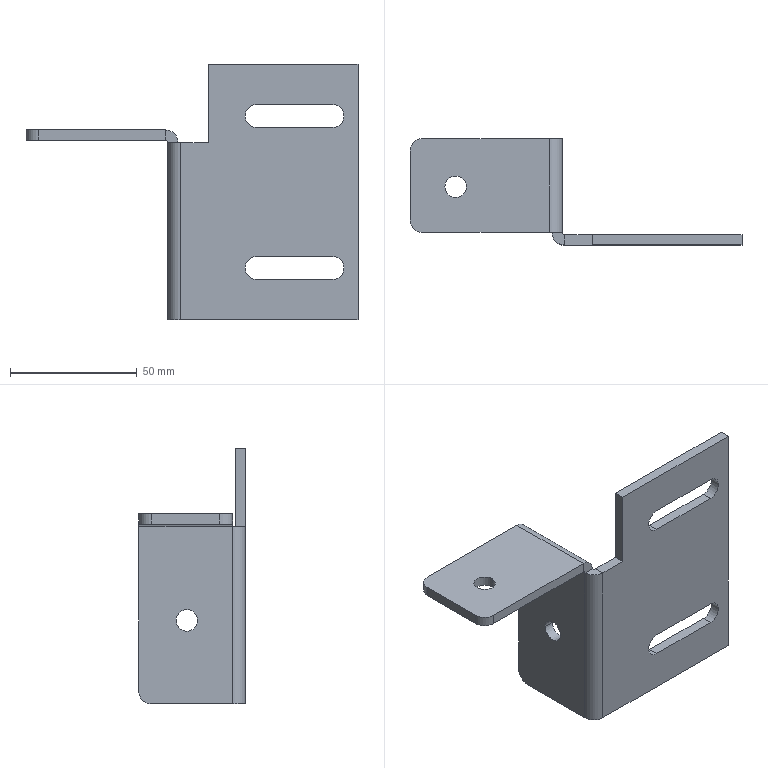Part | 1 solid | 39 faces | box 131 x 42 x 101 mm | volume 44246 mm3 | plane 24 | cylinder 15 | commonest cylinder face diameters 10 x5 8.5 x4 9 x4 2 x2
STEP:
#1=CARTESIAN_POINT('',(-24.207,-9.491,33.));
#2=VERTEX_POINT('',#1);
#3=CARTESIAN_POINT('',(-24.207,-0.9914,33.));
#4=VERTEX_POINT('',#3);
#5=CARTESIAN_POINT('',(-24.207,-5.241,33.));
#6=DIRECTION('',(1.,0.,0.));
#7=DIRECTION('',(0.,1.,0.));
#8=AXIS2_PLACEMENT_3D('',#5,#6,#7);
#9=CIRCLE('',#8,4.25);
#10=EDGE_CURVE('',#2,#4,#9,.T.);
#11=ORIENTED_EDGE('',*,*,#10,.F.);
#12=CARTESIAN_POINT('',(-20.207,-9.491,33.));
#13=VERTEX_POINT('',#12);
#14=CARTESIAN_POINT('',(-30.207,-9.491,33.));
#15=DIRECTION('',(1.,0.,0.));
#16=VECTOR('',#15,1000.);
#17=LINE('',#14,#16);
#18=EDGE_CURVE('',#2,#13,#17,.T.);
#19=ORIENTED_EDGE('',*,*,#18,.T.);
#20=CARTESIAN_POINT('',(-20.207,-0.9914,33.));
#21=VERTEX_POINT('',#20);
#22=CARTESIAN_POINT('',(-20.207,-5.241,33.));
#23=DIRECTION('',(1.,0.,0.));
#24=DIRECTION('',(0.,1.,0.));
#25=AXIS2_PLACEMENT_3D('',#22,#23,#24);
#26=CIRCLE('',#25,4.25);
#27=EDGE_CURVE('',#13,#21,#26,.T.);
#28=ORIENTED_EDGE('',*,*,#27,.T.);
#29=CARTESIAN_POINT('',(-30.207,-0.9914,33.));
#30=DIRECTION('',(1.,0.,0.));
#31=VECTOR('',#30,1000.);
#32=LINE('',#29,#31);
#33=EDGE_CURVE('',#4,#21,#32,.T.);
#34=ORIENTED_EDGE('',*,*,#33,.F.);
#35=EDGE_LOOP('',(#11,#19,#28,#34));
#36=FACE_OUTER_BOUND('',#35,.T.);
#37=CARTESIAN_POINT('',(-30.207,-5.241,33.));
#38=DIRECTION('',(1.,0.,0.));
#39=DIRECTION('',(0.,1.,0.));
#40=AXIS2_PLACEMENT_3D('',#37,#38,#39);
#41=CYLINDRICAL_SURFACE('',#40,4.25);
#42=ADVANCED_FACE('',(#36),#41,.F.);
#43=CARTESIAN_POINT('',(-66.457,-5.241,71.));
#44=VERTEX_POINT('',#43);
#45=CARTESIAN_POINT('',(-57.957,-5.241,71.));
#46=VERTEX_POINT('',#45);
#47=CARTESIAN_POINT('',(-62.207,-5.241,71.));
#48=DIRECTION('',(0.,0.,1.));
#49=DIRECTION('',(1.,0.,0.));
#50=AXIS2_PLACEMENT_3D('',#47,#48,#49);
#51=CIRCLE('',#50,4.25);
#52=EDGE_CURVE('',#44,#46,#51,.T.);
#53=ORIENTED_EDGE('',*,*,#52,.F.);
#54=CARTESIAN_POINT('',(-66.457,-5.241,75.));
#55=VERTEX_POINT('',#54);
#56=CARTESIAN_POINT('',(-66.457,-5.241,65.));
#57=DIRECTION('',(0.,0.,1.));
#58=VECTOR('',#57,1000.);
#59=LINE('',#56,#58);
#60=EDGE_CURVE('',#44,#55,#59,.T.);
#61=ORIENTED_EDGE('',*,*,#60,.T.);
#62=CARTESIAN_POINT('',(-57.957,-5.241,75.));
#63=VERTEX_POINT('',#62);
#64=CARTESIAN_POINT('',(-62.207,-5.241,75.));
#65=DIRECTION('',(0.,0.,1.));
#66=DIRECTION('',(1.,0.,0.));
#67=AXIS2_PLACEMENT_3D('',#64,#65,#66);
#68=CIRCLE('',#67,4.25);
#69=EDGE_CURVE('',#55,#63,#68,.T.);
#70=ORIENTED_EDGE('',*,*,#69,.T.);
#71=CARTESIAN_POINT('',(-57.957,-5.241,65.));
#72=DIRECTION('',(0.,0.,1.));
#73=VECTOR('',#72,1000.);
#74=LINE('',#71,#73);
#75=EDGE_CURVE('',#46,#63,#74,.T.);
#76=ORIENTED_EDGE('',*,*,#75,.F.);
#77=EDGE_LOOP('',(#53,#61,#70,#76));
#78=FACE_OUTER_BOUND('',#77,.T.);
#79=CARTESIAN_POINT('',(-62.207,-5.241,65.));
#80=DIRECTION('',(0.,0.,1.));
#81=DIRECTION('',(1.,0.,0.));
#82=AXIS2_PLACEMENT_3D('',#79,#80,#81);
#83=CYLINDRICAL_SURFACE('',#82,4.25);
#84=ADVANCED_FACE('',(#78),#83,.F.);
#85=CARTESIAN_POINT('',(-8.207,-24.241,70.));
#86=VERTEX_POINT('',#85);
#87=CARTESIAN_POINT('',(-19.207,-24.241,70.));
#88=VERTEX_POINT('',#87);
#89=CARTESIAN_POINT('',(-24.207,-24.241,70.));
#90=DIRECTION('',(-1.,0.,0.));
#91=VECTOR('',#90,1000.);
#92=LINE('',#89,#91);
#93=EDGE_CURVE('',#86,#88,#92,.T.);
#94=ORIENTED_EDGE('',*,*,#93,.T.);
#95=CARTESIAN_POINT('',(-19.207,-28.241,70.));
#96=VERTEX_POINT('',#95);
#97=CARTESIAN_POINT('',(-19.207,-24.241,70.));
#98=DIRECTION('',(0.,-1.,0.));
#99=VECTOR('',#98,1000.);
#100=LINE('',#97,#99);
#101=EDGE_CURVE('',#88,#96,#100,.T.);
#102=ORIENTED_EDGE('',*,*,#101,.T.);
#103=CARTESIAN_POINT('',(-8.207,-28.241,70.));
#104=VERTEX_POINT('',#103);
#105=CARTESIAN_POINT('',(-8.207,-28.241,70.));
#106=DIRECTION('',(-1.,0.,0.));
#107=VECTOR('',#106,1000.);
#108=LINE('',#105,#107);
#109=EDGE_CURVE('',#104,#96,#108,.T.);
#110=ORIENTED_EDGE('',*,*,#109,.F.);
#111=CARTESIAN_POINT('',(-8.207,-28.241,70.));
#112=DIRECTION('',(0.,1.,0.));
#113=VECTOR('',#112,1000.);
#114=LINE('',#111,#113);
#115=EDGE_CURVE('',#104,#86,#114,.T.);
#116=ORIENTED_EDGE('',*,*,#115,.T.);
#117=EDGE_LOOP('',(#94,#102,#110,#116));
#118=FACE_OUTER_BOUND('',#117,.T.);
#119=CARTESIAN_POINT('',(-8.207,-28.241,70.));
#120=DIRECTION('',(0.,0.,-1.));
#121=DIRECTION('',(-1.,0.,0.));
#122=AXIS2_PLACEMENT_3D('',#119,#120,#121);
#123=PLANE('',#122);
#124=ADVANCED_FACE('',(#118),#123,.F.);
#125=CARTESIAN_POINT('',(-19.207,-28.241,0.));
#126=VERTEX_POINT('',#125);
#127=CARTESIAN_POINT('',(-19.207,-24.241,0.));
#128=VERTEX_POINT('',#127);
#129=CARTESIAN_POINT('',(-19.207,-28.241,0.));
#130=DIRECTION('',(0.,1.,0.));
#131=VECTOR('',#130,1000.);
#132=LINE('',#129,#131);
#133=EDGE_CURVE('',#126,#128,#132,.T.);
#134=ORIENTED_EDGE('',*,*,#133,.F.);
#135=CARTESIAN_POINT('',(-24.207,-23.241,0.));
#136=VERTEX_POINT('',#135);
#137=CARTESIAN_POINT('',(-19.207,-23.241,0.));
#138=DIRECTION('',(0.,0.,1.));
#139=DIRECTION('',(-1.,0.,0.));
#140=AXIS2_PLACEMENT_3D('',#137,#138,#139);
#141=CIRCLE('',#140,5.);
#142=EDGE_CURVE('',#136,#126,#141,.T.);
#143=ORIENTED_EDGE('',*,*,#142,.F.);
#144=CARTESIAN_POINT('',(-20.207,-23.241,0.));
#145=VERTEX_POINT('',#144);
#146=CARTESIAN_POINT('',(-20.207,-23.241,0.));
#147=DIRECTION('',(-1.,0.,0.));
#148=VECTOR('',#147,1000.);
#149=LINE('',#146,#148);
#150=EDGE_CURVE('',#145,#136,#149,.T.);
#151=ORIENTED_EDGE('',*,*,#150,.F.);
#152=CARTESIAN_POINT('',(-19.207,-23.241,0.));
#153=DIRECTION('',(0.,0.,1.));
#154=DIRECTION('',(1.,0.,0.));
#155=AXIS2_PLACEMENT_3D('',#152,#153,#154);
#156=CIRCLE('',#155,1.);
#157=EDGE_CURVE('',#145,#128,#156,.T.);
#158=ORIENTED_EDGE('',*,*,#157,.T.);
#159=EDGE_LOOP('',(#134,#143,#151,#158));
#160=FACE_OUTER_BOUND('',#159,.T.);
#161=CARTESIAN_POINT('',(-19.207,-28.241,0.));
#162=DIRECTION('',(0.,0.,-1.));
#163=DIRECTION('',(-1.,0.,0.));
#164=AXIS2_PLACEMENT_3D('',#161,#162,#163);
#165=PLANE('',#164);
#166=ADVANCED_FACE('',(#160),#165,.T.);
#167=CARTESIAN_POINT('',(50.793,-28.241,0.));
#168=VERTEX_POINT('',#167);
#169=CARTESIAN_POINT('',(50.793,-24.241,0.));
#170=VERTEX_POINT('',#169);
#171=CARTESIAN_POINT('',(50.793,-34.241,0.));
#172=DIRECTION('',(0.,1.,0.));
#173=VECTOR('',#172,1000.);
#174=LINE('',#171,#173);
#175=EDGE_CURVE('',#168,#170,#174,.T.);
#176=ORIENTED_EDGE('',*,*,#175,.F.);
#177=CARTESIAN_POINT('',(-24.207,-28.241,0.));
#178=DIRECTION('',(1.,0.,0.));
#179=VECTOR('',#178,1000.);
#180=LINE('',#177,#179);
#181=EDGE_CURVE('',#126,#168,#180,.T.);
#182=ORIENTED_EDGE('',*,*,#181,.F.);
#183=ORIENTED_EDGE('',*,*,#133,.T.);
#184=CARTESIAN_POINT('',(-24.207,-24.241,0.));
#185=DIRECTION('',(1.,0.,0.));
#186=VECTOR('',#185,1000.);
#187=LINE('',#184,#186);
#188=EDGE_CURVE('',#128,#170,#187,.T.);
#189=ORIENTED_EDGE('',*,*,#188,.T.);
#190=EDGE_LOOP('',(#176,#182,#183,#189));
#191=FACE_OUTER_BOUND('',#190,.T.);
#192=CARTESIAN_POINT('',(-20.207,-23.241,0.));
#193=DIRECTION('',(0.,0.,-1.));
#194=DIRECTION('',(-1.,0.,0.));
#195=AXIS2_PLACEMENT_3D('',#192,#193,#194);
#196=PLANE('',#195);
#197=ADVANCED_FACE('',(#191),#196,.T.);
#198=CARTESIAN_POINT('',(40.793,-28.241,16.));
#199=VERTEX_POINT('',#198);
#200=CARTESIAN_POINT('',(10.793,-28.241,16.));
#201=VERTEX_POINT('',#200);
#202=CARTESIAN_POINT('',(-24.207,-28.241,16.));
#203=DIRECTION('',(-1.,0.,0.));
#204=VECTOR('',#203,1000.);
#205=LINE('',#202,#204);
#206=EDGE_CURVE('',#199,#201,#205,.T.);
#207=ORIENTED_EDGE('',*,*,#206,.T.);
#208=CARTESIAN_POINT('',(10.793,-28.241,25.));
#209=VERTEX_POINT('',#208);
#210=CARTESIAN_POINT('',(10.793,-28.241,20.5));
#211=DIRECTION('',(0.,1.,0.));
#212=DIRECTION('',(0.,0.,1.));
#213=AXIS2_PLACEMENT_3D('',#210,#211,#212);
#214=CIRCLE('',#213,4.5);
#215=EDGE_CURVE('',#201,#209,#214,.T.);
#216=ORIENTED_EDGE('',*,*,#215,.T.);
#217=CARTESIAN_POINT('',(40.793,-28.241,25.));
#218=VERTEX_POINT('',#217);
#219=CARTESIAN_POINT('',(-24.207,-28.241,25.));
#220=DIRECTION('',(1.,0.,0.));
#221=VECTOR('',#220,1000.);
#222=LINE('',#219,#221);
#223=EDGE_CURVE('',#209,#218,#222,.T.);
#224=ORIENTED_EDGE('',*,*,#223,.T.);
#225=CARTESIAN_POINT('',(40.793,-28.241,20.5));
#226=DIRECTION('',(0.,1.,0.));
#227=DIRECTION('',(0.,0.,1.));
#228=AXIS2_PLACEMENT_3D('',#225,#226,#227);
#229=CIRCLE('',#228,4.5);
#230=EDGE_CURVE('',#218,#199,#229,.T.);
#231=ORIENTED_EDGE('',*,*,#230,.T.);
#232=EDGE_LOOP('',(#207,#216,#224,#231));
#233=FACE_BOUND('',#232,.T.);
#234=CARTESIAN_POINT('',(40.793,-28.241,76.));
#235=VERTEX_POINT('',#234);
#236=CARTESIAN_POINT('',(10.793,-28.241,76.));
#237=VERTEX_POINT('',#236);
#238=CARTESIAN_POINT('',(-24.207,-28.241,76.));
#239=DIRECTION('',(-1.,0.,0.));
#240=VECTOR('',#239,1000.);
#241=LINE('',#238,#240);
#242=EDGE_CURVE('',#235,#237,#241,.T.);
#243=ORIENTED_EDGE('',*,*,#242,.T.);
#244=CARTESIAN_POINT('',(10.793,-28.241,85.));
#245=VERTEX_POINT('',#244);
#246=CARTESIAN_POINT('',(10.793,-28.241,80.5));
#247=DIRECTION('',(0.,1.,0.));
#248=DIRECTION('',(0.,0.,1.));
#249=AXIS2_PLACEMENT_3D('',#246,#247,#248);
#250=CIRCLE('',#249,4.5);
#251=EDGE_CURVE('',#237,#245,#250,.T.);
#252=ORIENTED_EDGE('',*,*,#251,.T.);
#253=CARTESIAN_POINT('',(40.793,-28.241,85.));
#254=VERTEX_POINT('',#253);
#255=CARTESIAN_POINT('',(-24.207,-28.241,85.));
#256=DIRECTION('',(1.,0.,0.));
#257=VECTOR('',#256,1000.);
#258=LINE('',#255,#257);
#259=EDGE_CURVE('',#245,#254,#258,.T.);
#260=ORIENTED_EDGE('',*,*,#259,.T.);
#261=CARTESIAN_POINT('',(40.793,-28.241,80.5));
#262=DIRECTION('',(0.,1.,0.));
#263=DIRECTION('',(0.,0.,1.));
#264=AXIS2_PLACEMENT_3D('',#261,#262,#263);
#265=CIRCLE('',#264,4.5);
#266=EDGE_CURVE('',#254,#235,#265,.T.);
#267=ORIENTED_EDGE('',*,*,#266,.T.);
#268=EDGE_LOOP('',(#243,#252,#260,#267));
#269=FACE_BOUND('',#268,.T.);
#270=ORIENTED_EDGE('',*,*,#181,.T.);
#271=CARTESIAN_POINT('',(50.793,-28.241,101.));
#272=VERTEX_POINT('',#271);
#273=CARTESIAN_POINT('',(50.793,-28.241,125.));
#274=DIRECTION('',(0.,0.,1.));
#275=VECTOR('',#274,1000.);
#276=LINE('',#273,#275);
#277=EDGE_CURVE('',#168,#272,#276,.T.);
#278=ORIENTED_EDGE('',*,*,#277,.T.);
#279=CARTESIAN_POINT('',(-8.207,-28.241,101.));
#280=VERTEX_POINT('',#279);
#281=CARTESIAN_POINT('',(-24.207,-28.241,101.));
#282=DIRECTION('',(-1.,0.,0.));
#283=VECTOR('',#282,1000.);
#284=LINE('',#281,#283);
#285=EDGE_CURVE('',#272,#280,#284,.T.);
#286=ORIENTED_EDGE('',*,*,#285,.T.);
#287=CARTESIAN_POINT('',(-8.207,-28.241,125.));
#288=DIRECTION('',(0.,0.,-1.));
#289=VECTOR('',#288,1000.);
#290=LINE('',#287,#289);
#291=EDGE_CURVE('',#280,#104,#290,.T.);
#292=ORIENTED_EDGE('',*,*,#291,.T.);
#293=ORIENTED_EDGE('',*,*,#109,.T.);
#294=CARTESIAN_POINT('',(-19.207,-28.241,125.));
#295=DIRECTION('',(0.,0.,-1.));
#296=VECTOR('',#295,1000.);
#297=LINE('',#294,#296);
#298=EDGE_CURVE('',#96,#126,#297,.T.);
#299=ORIENTED_EDGE('',*,*,#298,.T.);
#300=EDGE_LOOP('',(#270,#278,#286,#292,#293,#299));
#301=FACE_OUTER_BOUND('',#300,.T.);
#302=CARTESIAN_POINT('',(-24.207,-28.241,125.));
#303=DIRECTION('',(0.,1.,0.));
#304=DIRECTION('',(0.,0.,1.));
#305=AXIS2_PLACEMENT_3D('',#302,#303,#304);
#306=PLANE('',#305);
#307=ADVANCED_FACE('',(#233,#269,#301),#306,.F.);
#308=CARTESIAN_POINT('',(10.793,-24.241,16.));
#309=VERTEX_POINT('',#308);
#310=CARTESIAN_POINT('',(10.793,-24.241,25.));
#311=VERTEX_POINT('',#310);
#312=CARTESIAN_POINT('',(10.793,-24.241,20.5));
#313=DIRECTION('',(0.,1.,0.));
#314=DIRECTION('',(0.,0.,1.));
#315=AXIS2_PLACEMENT_3D('',#312,#313,#314);
#316=CIRCLE('',#315,4.5);
#317=EDGE_CURVE('',#309,#311,#316,.T.);
#318=ORIENTED_EDGE('',*,*,#317,.F.);
#319=CARTESIAN_POINT('',(40.793,-24.241,16.));
#320=VERTEX_POINT('',#319);
#321=CARTESIAN_POINT('',(10.793,-24.241,16.));
#322=DIRECTION('',(-1.,0.,0.));
#323=VECTOR('',#322,1000.);
#324=LINE('',#321,#323);
#325=EDGE_CURVE('',#320,#309,#324,.T.);
#326=ORIENTED_EDGE('',*,*,#325,.F.);
#327=CARTESIAN_POINT('',(40.793,-24.241,25.));
#328=VERTEX_POINT('',#327);
#329=CARTESIAN_POINT('',(40.793,-24.241,20.5));
#330=DIRECTION('',(0.,1.,0.));
#331=DIRECTION('',(0.,0.,1.));
#332=AXIS2_PLACEMENT_3D('',#329,#330,#331);
#333=CIRCLE('',#332,4.5);
#334=EDGE_CURVE('',#328,#320,#333,.T.);
#335=ORIENTED_EDGE('',*,*,#334,.F.);
#336=CARTESIAN_POINT('',(10.793,-24.241,25.));
#337=DIRECTION('',(1.,0.,0.));
#338=VECTOR('',#337,1000.);
#339=LINE('',#336,#338);
#340=EDGE_CURVE('',#311,#328,#339,.T.);
#341=ORIENTED_EDGE('',*,*,#340,.F.);
#342=EDGE_LOOP('',(#318,#326,#335,#341));
#343=FACE_BOUND('',#342,.T.);
#344=CARTESIAN_POINT('',(10.793,-24.241,76.));
#345=VERTEX_POINT('',#344);
#346=CARTESIAN_POINT('',(10.793,-24.241,85.));
#347=VERTEX_POINT('',#346);
#348=CARTESIAN_POINT('',(10.793,-24.241,80.5));
#349=DIRECTION('',(0.,1.,0.));
#350=DIRECTION('',(0.,0.,-1.));
#351=AXIS2_PLACEMENT_3D('',#348,#349,#350);
#352=CIRCLE('',#351,4.5);
#353=EDGE_CURVE('',#345,#347,#352,.T.);
#354=ORIENTED_EDGE('',*,*,#353,.F.);
#355=CARTESIAN_POINT('',(40.793,-24.241,76.));
#356=VERTEX_POINT('',#355);
#357=CARTESIAN_POINT('',(10.793,-24.241,76.));
#358=DIRECTION('',(-1.,0.,0.));
#359=VECTOR('',#358,1000.);
#360=LINE('',#357,#359);
#361=EDGE_CURVE('',#356,#345,#360,.T.);
#362=ORIENTED_EDGE('',*,*,#361,.F.);
#363=CARTESIAN_POINT('',(40.793,-24.241,85.));
#364=VERTEX_POINT('',#363);
#365=CARTESIAN_POINT('',(40.793,-24.241,80.5));
#366=DIRECTION('',(0.,1.,0.));
#367=DIRECTION('',(0.,0.,-1.));
#368=AXIS2_PLACEMENT_3D('',#365,#366,#367);
#369=CIRCLE('',#368,4.5);
#370=EDGE_CURVE('',#364,#356,#369,.T.);
#371=ORIENTED_EDGE('',*,*,#370,.F.);
#372=CARTESIAN_POINT('',(10.793,-24.241,85.));
#373=DIRECTION('',(1.,0.,0.));
#374=VECTOR('',#373,1000.);
#375=LINE('',#372,#374);
#376=EDGE_CURVE('',#347,#364,#375,.T.);
#377=ORIENTED_EDGE('',*,*,#376,.F.);
#378=EDGE_LOOP('',(#354,#362,#371,#377));
#379=FACE_BOUND('',#378,.T.);
#380=CARTESIAN_POINT('',(50.793,-24.241,101.));
#381=VERTEX_POINT('',#380);
#382=CARTESIAN_POINT('',(50.793,-24.241,0.));
#383=DIRECTION('',(0.,0.,1.));
#384=VECTOR('',#383,1000.);
#385=LINE('',#382,#384);
#386=EDGE_CURVE('',#170,#381,#385,.T.);
#387=ORIENTED_EDGE('',*,*,#386,.F.);
#388=ORIENTED_EDGE('',*,*,#188,.F.);
#389=CARTESIAN_POINT('',(-19.207,-24.241,125.));
#390=DIRECTION('',(0.,0.,-1.));
#391=VECTOR('',#390,1000.);
#392=LINE('',#389,#391);
#393=EDGE_CURVE('',#88,#128,#392,.T.);
#394=ORIENTED_EDGE('',*,*,#393,.F.);
#395=ORIENTED_EDGE('',*,*,#93,.F.);
#396=CARTESIAN_POINT('',(-8.207,-24.241,101.));
#397=VERTEX_POINT('',#396);
#398=CARTESIAN_POINT('',(-8.207,-24.241,125.));
#399=DIRECTION('',(0.,0.,-1.));
#400=VECTOR('',#399,1000.);
#401=LINE('',#398,#400);
#402=EDGE_CURVE('',#397,#86,#401,.T.);
#403=ORIENTED_EDGE('',*,*,#402,.F.);
#404=CARTESIAN_POINT('',(-8.207,-24.241,101.));
#405=DIRECTION('',(-1.,0.,0.));
#406=VECTOR('',#405,1000.);
#407=LINE('',#404,#406);
#408=EDGE_CURVE('',#381,#397,#407,.T.);
#409=ORIENTED_EDGE('',*,*,#408,.F.);
#410=EDGE_LOOP('',(#387,#388,#394,#395,#403,#409));
#411=FACE_OUTER_BOUND('',#410,.T.);
#412=CARTESIAN_POINT('',(-24.207,-24.241,125.));
#413=DIRECTION('',(0.,1.,0.));
#414=DIRECTION('',(0.,0.,1.));
#415=AXIS2_PLACEMENT_3D('',#412,#413,#414);
#416=PLANE('',#415);
#417=ADVANCED_FACE('',(#343,#379,#411),#416,.T.);
#418=CARTESIAN_POINT('',(-20.207,-23.241,70.));
#419=VERTEX_POINT('',#418);
#420=CARTESIAN_POINT('',(-19.207,-23.241,70.));
#421=DIRECTION('',(0.,0.,-1.));
#422=DIRECTION('',(-1.,0.,0.));
#423=AXIS2_PLACEMENT_3D('',#420,#421,#422);
#424=CIRCLE('',#423,1.);
#425=EDGE_CURVE('',#88,#419,#424,.T.);
#426=ORIENTED_EDGE('',*,*,#425,.F.);
#427=ORIENTED_EDGE('',*,*,#393,.T.);
#428=ORIENTED_EDGE('',*,*,#157,.F.);
#429=CARTESIAN_POINT('',(-20.207,-23.241,125.));
#430=DIRECTION('',(0.,0.,-1.));
#431=VECTOR('',#430,1000.);
#432=LINE('',#429,#431);
#433=EDGE_CURVE('',#419,#145,#432,.T.);
#434=ORIENTED_EDGE('',*,*,#433,.F.);
#435=EDGE_LOOP('',(#426,#427,#428,#434));
#436=FACE_OUTER_BOUND('',#435,.T.);
#437=CARTESIAN_POINT('',(-19.207,-23.241,125.));
#438=DIRECTION('',(0.,0.,-1.));
#439=DIRECTION('',(-1.,0.,0.));
#440=AXIS2_PLACEMENT_3D('',#437,#438,#439);
#441=CYLINDRICAL_SURFACE('',#440,1.);
#442=ADVANCED_FACE('',(#436),#441,.F.);
#443=CARTESIAN_POINT('',(-20.207,-5.241,33.));
#444=DIRECTION('',(1.,0.,0.));
#445=DIRECTION('',(0.,1.,0.));
#446=AXIS2_PLACEMENT_3D('',#443,#444,#445);
#447=CIRCLE('',#446,4.25);
#448=EDGE_CURVE('',#21,#13,#447,.T.);
#449=ORIENTED_EDGE('',*,*,#448,.F.);
#450=ORIENTED_EDGE('',*,*,#27,.F.);
#451=EDGE_LOOP('',(#449,#450));
#452=FACE_BOUND('',#451,.T.);
#453=CARTESIAN_POINT('',(-20.207,8.759,0.));
#454=VERTEX_POINT('',#453);
#455=CARTESIAN_POINT('',(-20.207,13.759,0.));
#456=DIRECTION('',(0.,-1.,0.));
#457=VECTOR('',#456,1000.);
#458=LINE('',#455,#457);
#459=EDGE_CURVE('',#454,#145,#458,.T.);
#460=ORIENTED_EDGE('',*,*,#459,.F.);
#461=CARTESIAN_POINT('',(-20.207,13.759,5.));
#462=VERTEX_POINT('',#461);
#463=CARTESIAN_POINT('',(-20.207,8.759,5.));
#464=DIRECTION('',(1.,0.,0.));
#465=DIRECTION('',(0.,1.,0.));
#466=AXIS2_PLACEMENT_3D('',#463,#464,#465);
#467=CIRCLE('',#466,5.);
#468=EDGE_CURVE('',#454,#462,#467,.T.);
#469=ORIENTED_EDGE('',*,*,#468,.T.);
#470=CARTESIAN_POINT('',(-20.207,13.759,70.));
#471=VERTEX_POINT('',#470);
#472=CARTESIAN_POINT('',(-20.207,13.759,125.));
#473=DIRECTION('',(0.,0.,-1.));
#474=VECTOR('',#473,1000.);
#475=LINE('',#472,#474);
#476=EDGE_CURVE('',#471,#462,#475,.T.);
#477=ORIENTED_EDGE('',*,*,#476,.F.);
#478=CARTESIAN_POINT('',(-20.207,13.759,70.));
#479=DIRECTION('',(0.,1.,0.));
#480=VECTOR('',#479,1000.);
#481=LINE('',#478,#480);
#482=EDGE_CURVE('',#419,#471,#481,.T.);
#483=ORIENTED_EDGE('',*,*,#482,.F.);
#484=ORIENTED_EDGE('',*,*,#433,.T.);
#485=EDGE_LOOP('',(#460,#469,#477,#483,#484));
#486=FACE_OUTER_BOUND('',#485,.T.);
#487=CARTESIAN_POINT('',(-20.207,13.759,125.));
#488=DIRECTION('',(1.,0.,0.));
#489=DIRECTION('',(0.,1.,0.));
#490=AXIS2_PLACEMENT_3D('',#487,#488,#489);
#491=PLANE('',#490);
#492=ADVANCED_FACE('',(#452,#486),#491,.T.);
#493=ORIENTED_EDGE('',*,*,#476,.T.);
#494=CARTESIAN_POINT('',(-24.207,13.759,5.));
#495=VERTEX_POINT('',#494);
#496=CARTESIAN_POINT('',(-24.207,13.759,5.));
#497=DIRECTION('',(-1.,0.,0.));
#498=VECTOR('',#497,1000.);
#499=LINE('',#496,#498);
#500=EDGE_CURVE('',#462,#495,#499,.T.);
#501=ORIENTED_EDGE('',*,*,#500,.T.);
#502=CARTESIAN_POINT('',(-24.207,13.759,70.));
#503=VERTEX_POINT('',#502);
#504=CARTESIAN_POINT('',(-24.207,13.759,125.));
#505=DIRECTION('',(0.,0.,-1.));
#506=VECTOR('',#505,1000.);
#507=LINE('',#504,#506);
#508=EDGE_CURVE('',#503,#495,#507,.T.);
#509=ORIENTED_EDGE('',*,*,#508,.F.);
#510=CARTESIAN_POINT('',(-8.207,13.759,70.));
#511=DIRECTION('',(-1.,0.,0.));
#512=VECTOR('',#511,1000.);
#513=LINE('',#510,#512);
#514=EDGE_CURVE('',#471,#503,#513,.T.);
#515=ORIENTED_EDGE('',*,*,#514,.F.);
#516=EDGE_LOOP('',(#493,#501,#509,#515));
#517=FACE_OUTER_BOUND('',#516,.T.);
#518=CARTESIAN_POINT('',(-24.207,13.759,125.));
#519=DIRECTION('',(0.,1.,0.));
#520=DIRECTION('',(0.,0.,1.));
#521=AXIS2_PLACEMENT_3D('',#518,#519,#520);
#522=PLANE('',#521);
#523=ADVANCED_FACE('',(#517),#522,.T.);
#524=CARTESIAN_POINT('',(-24.207,-5.241,33.));
#525=DIRECTION('',(1.,0.,0.));
#526=DIRECTION('',(0.,1.,0.));
#527=AXIS2_PLACEMENT_3D('',#524,#525,#526);
#528=CIRCLE('',#527,4.25);
#529=EDGE_CURVE('',#4,#2,#528,.T.);
#530=ORIENTED_EDGE('',*,*,#529,.T.);
#531=ORIENTED_EDGE('',*,*,#10,.T.);
#532=EDGE_LOOP('',(#530,#531));
#533=FACE_BOUND('',#532,.T.);
#534=ORIENTED_EDGE('',*,*,#508,.T.);
#535=CARTESIAN_POINT('',(-24.207,8.759,0.));
#536=VERTEX_POINT('',#535);
#537=CARTESIAN_POINT('',(-24.207,8.759,5.));
#538=DIRECTION('',(-1.,0.,0.));
#539=DIRECTION('',(0.,1.,0.));
#540=AXIS2_PLACEMENT_3D('',#537,#538,#539);
#541=CIRCLE('',#540,5.);
#542=EDGE_CURVE('',#495,#536,#541,.T.);
#543=ORIENTED_EDGE('',*,*,#542,.T.);
#544=CARTESIAN_POINT('',(-24.207,13.759,0.));
#545=DIRECTION('',(0.,-1.,0.));
#546=VECTOR('',#545,1000.);
#547=LINE('',#544,#546);
#548=EDGE_CURVE('',#536,#136,#547,.T.);
#549=ORIENTED_EDGE('',*,*,#548,.T.);
#550=CARTESIAN_POINT('',(-24.207,-23.241,70.));
#551=VERTEX_POINT('',#550);
#552=CARTESIAN_POINT('',(-24.207,-23.241,125.));
#553=DIRECTION('',(0.,0.,-1.));
#554=VECTOR('',#553,1000.);
#555=LINE('',#552,#554);
#556=EDGE_CURVE('',#551,#136,#555,.T.);
#557=ORIENTED_EDGE('',*,*,#556,.F.);
#558=CARTESIAN_POINT('',(-24.207,13.759,70.));
#559=DIRECTION('',(0.,1.,0.));
#560=VECTOR('',#559,1000.);
#561=LINE('',#558,#560);
#562=EDGE_CURVE('',#551,#503,#561,.T.);
#563=ORIENTED_EDGE('',*,*,#562,.T.);
#564=EDGE_LOOP('',(#534,#543,#549,#557,#563));
#565=FACE_OUTER_BOUND('',#564,.T.);
#566=CARTESIAN_POINT('',(-24.207,13.759,125.));
#567=DIRECTION('',(1.,0.,0.));
#568=DIRECTION('',(0.,1.,0.));
#569=AXIS2_PLACEMENT_3D('',#566,#567,#568);
#570=PLANE('',#569);
#571=ADVANCED_FACE('',(#533,#565),#570,.F.);
#572=ORIENTED_EDGE('',*,*,#298,.F.);
#573=CARTESIAN_POINT('',(-19.207,-23.241,70.));
#574=DIRECTION('',(0.,0.,-1.));
#575=DIRECTION('',(-1.,0.,0.));
#576=AXIS2_PLACEMENT_3D('',#573,#574,#575);
#577=CIRCLE('',#576,5.);
#578=EDGE_CURVE('',#96,#551,#577,.T.);
#579=ORIENTED_EDGE('',*,*,#578,.T.);
#580=ORIENTED_EDGE('',*,*,#556,.T.);
#581=ORIENTED_EDGE('',*,*,#142,.T.);
#582=EDGE_LOOP('',(#572,#579,#580,#581));
#583=FACE_OUTER_BOUND('',#582,.T.);
#584=CARTESIAN_POINT('',(-19.207,-23.241,125.));
#585=DIRECTION('',(0.,0.,-1.));
#586=DIRECTION('',(-1.,0.,0.));
#587=AXIS2_PLACEMENT_3D('',#584,#585,#586);
#588=CYLINDRICAL_SURFACE('',#587,5.);
#589=ADVANCED_FACE('',(#583),#588,.T.);
#590=ORIENTED_EDGE('',*,*,#548,.F.);
#591=CARTESIAN_POINT('',(-20.207,8.759,0.));
#592=DIRECTION('',(1.,0.,0.));
#593=VECTOR('',#592,1000.);
#594=LINE('',#591,#593);
#595=EDGE_CURVE('',#536,#454,#594,.T.);
#596=ORIENTED_EDGE('',*,*,#595,.T.);
#597=ORIENTED_EDGE('',*,*,#459,.T.);
#598=ORIENTED_EDGE('',*,*,#150,.T.);
#599=EDGE_LOOP('',(#590,#596,#597,#598));
#600=FACE_OUTER_BOUND('',#599,.T.);
#601=CARTESIAN_POINT('',(-19.207,-23.241,0.));
#602=DIRECTION('',(0.,0.,1.));
#603=DIRECTION('',(1.,0.,0.));
#604=AXIS2_PLACEMENT_3D('',#601,#602,#603);
#605=PLANE('',#604);
#606=ADVANCED_FACE('',(#600),#605,.F.);
#607=CARTESIAN_POINT('',(-24.207,-23.241,70.));
#608=DIRECTION('',(1.,0.,0.));
#609=VECTOR('',#608,1000.);
#610=LINE('',#607,#609);
#611=EDGE_CURVE('',#551,#419,#610,.T.);
#612=ORIENTED_EDGE('',*,*,#611,.F.);
#613=ORIENTED_EDGE('',*,*,#578,.F.);
#614=ORIENTED_EDGE('',*,*,#101,.F.);
#615=ORIENTED_EDGE('',*,*,#425,.T.);
#616=EDGE_LOOP('',(#612,#613,#614,#615));
#617=FACE_OUTER_BOUND('',#616,.T.);
#618=CARTESIAN_POINT('',(-8.207,-28.241,70.));
#619=DIRECTION('',(0.,0.,-1.));
#620=DIRECTION('',(-1.,0.,0.));
#621=AXIS2_PLACEMENT_3D('',#618,#619,#620);
#622=PLANE('',#621);
#623=ADVANCED_FACE('',(#617),#622,.F.);
#624=ORIENTED_EDGE('',*,*,#291,.F.);
#625=CARTESIAN_POINT('',(-8.207,-28.241,101.));
#626=DIRECTION('',(0.,1.,0.));
#627=VECTOR('',#626,1000.);
#628=LINE('',#625,#627);
#629=EDGE_CURVE('',#280,#397,#628,.T.);
#630=ORIENTED_EDGE('',*,*,#629,.T.);
#631=ORIENTED_EDGE('',*,*,#402,.T.);
#632=ORIENTED_EDGE('',*,*,#115,.F.);
#633=EDGE_LOOP('',(#624,#630,#631,#632));
#634=FACE_OUTER_BOUND('',#633,.T.);
#635=CARTESIAN_POINT('',(-8.207,-28.241,125.));
#636=DIRECTION('',(1.,0.,0.));
#637=DIRECTION('',(0.,0.,-1.));
#638=AXIS2_PLACEMENT_3D('',#635,#636,#637);
#639=PLANE('',#638);
#640=ADVANCED_FACE('',(#634),#639,.F.);
#641=CARTESIAN_POINT('',(-25.207,-23.241,71.));
#642=VERTEX_POINT('',#641);
#643=CARTESIAN_POINT('',(-25.207,-23.241,75.));
#644=VERTEX_POINT('',#643);
#645=CARTESIAN_POINT('',(-25.207,-23.241,75.));
#646=DIRECTION('',(0.,0.,1.));
#647=VECTOR('',#646,1000.);
#648=LINE('',#645,#647);
#649=EDGE_CURVE('',#642,#644,#648,.T.);
#650=ORIENTED_EDGE('',*,*,#649,.F.);
#651=CARTESIAN_POINT('',(-25.207,-23.241,70.));
#652=DIRECTION('',(0.,-1.,0.));
#653=DIRECTION('',(0.,0.,1.));
#654=AXIS2_PLACEMENT_3D('',#651,#652,#653);
#655=CIRCLE('',#654,1.);
#656=EDGE_CURVE('',#551,#642,#655,.T.);
#657=ORIENTED_EDGE('',*,*,#656,.F.);
#658=ORIENTED_EDGE('',*,*,#611,.T.);
#659=CARTESIAN_POINT('',(-25.207,-23.241,70.));
#660=DIRECTION('',(0.,-1.,0.));
#661=DIRECTION('',(0.,0.,1.));
#662=AXIS2_PLACEMENT_3D('',#659,#660,#661);
#663=CIRCLE('',#662,5.);
#664=EDGE_CURVE('',#419,#644,#663,.T.);
#665=ORIENTED_EDGE('',*,*,#664,.T.);
#666=EDGE_LOOP('',(#650,#657,#658,#665));
#667=FACE_OUTER_BOUND('',#666,.T.);
#668=CARTESIAN_POINT('',(-25.207,-23.241,70.));
#669=DIRECTION('',(0.,-1.,0.));
#670=DIRECTION('',(0.,0.,-1.));
#671=AXIS2_PLACEMENT_3D('',#668,#669,#670);
#672=PLANE('',#671);
#673=ADVANCED_FACE('',(#667),#672,.T.);
#674=CARTESIAN_POINT('',(-25.207,13.759,71.));
#675=VERTEX_POINT('',#674);
#676=CARTESIAN_POINT('',(-25.207,13.759,70.));
#677=DIRECTION('',(0.,1.,0.));
#678=DIRECTION('',(0.,0.,1.));
#679=AXIS2_PLACEMENT_3D('',#676,#677,#678);
#680=CIRCLE('',#679,1.);
#681=EDGE_CURVE('',#675,#503,#680,.T.);
#682=ORIENTED_EDGE('',*,*,#681,.F.);
#683=CARTESIAN_POINT('',(-25.207,13.759,75.));
#684=VERTEX_POINT('',#683);
#685=CARTESIAN_POINT('',(-25.207,13.759,71.));
#686=DIRECTION('',(0.,0.,1.));
#687=VECTOR('',#686,1000.);
#688=LINE('',#685,#687);
#689=EDGE_CURVE('',#675,#684,#688,.T.);
#690=ORIENTED_EDGE('',*,*,#689,.T.);
#691=CARTESIAN_POINT('',(-25.207,13.759,70.));
#692=DIRECTION('',(0.,1.,0.));
#693=DIRECTION('',(0.,0.,1.));
#694=AXIS2_PLACEMENT_3D('',#691,#692,#693);
#695=CIRCLE('',#694,5.);
#696=EDGE_CURVE('',#684,#471,#695,.T.);
#697=ORIENTED_EDGE('',*,*,#696,.T.);
#698=ORIENTED_EDGE('',*,*,#514,.T.);
#699=EDGE_LOOP('',(#682,#690,#697,#698));
#700=FACE_OUTER_BOUND('',#699,.T.);
#701=CARTESIAN_POINT('',(-25.207,13.759,70.));
#702=DIRECTION('',(0.,-1.,0.));
#703=DIRECTION('',(0.,0.,-1.));
#704=AXIS2_PLACEMENT_3D('',#701,#702,#703);
#705=PLANE('',#704);
#706=ADVANCED_FACE('',(#700),#705,.F.);
#707=ORIENTED_EDGE('',*,*,#482,.T.);
#708=ORIENTED_EDGE('',*,*,#696,.F.);
#709=CARTESIAN_POINT('',(-25.207,0.,75.));
#710=DIRECTION('',(0.,1.,0.));
#711=VECTOR('',#710,1000.);
#712=LINE('',#709,#711);
#713=EDGE_CURVE('',#644,#684,#712,.T.);
#714=ORIENTED_EDGE('',*,*,#713,.F.);
#715=ORIENTED_EDGE('',*,*,#664,.F.);
#716=EDGE_LOOP('',(#707,#708,#714,#715));
#717=FACE_OUTER_BOUND('',#716,.T.);
#718=CARTESIAN_POINT('',(-25.207,13.759,70.));
#719=DIRECTION('',(0.,1.,0.));
#720=DIRECTION('',(0.,0.,1.));
#721=AXIS2_PLACEMENT_3D('',#718,#719,#720);
#722=CYLINDRICAL_SURFACE('',#721,5.);
#723=ADVANCED_FACE('',(#717),#722,.T.);
#724=ORIENTED_EDGE('',*,*,#562,.F.);
#725=ORIENTED_EDGE('',*,*,#656,.T.);
#726=CARTESIAN_POINT('',(-25.207,-23.241,71.));
#727=DIRECTION('',(0.,1.,0.));
#728=VECTOR('',#727,1000.);
#729=LINE('',#726,#728);
#730=EDGE_CURVE('',#642,#675,#729,.T.);
#731=ORIENTED_EDGE('',*,*,#730,.T.);
#732=ORIENTED_EDGE('',*,*,#681,.T.);
#733=EDGE_LOOP('',(#724,#725,#731,#732));
#734=FACE_OUTER_BOUND('',#733,.T.);
#735=CARTESIAN_POINT('',(-25.207,13.759,70.));
#736=DIRECTION('',(0.,1.,0.));
#737=DIRECTION('',(0.,0.,1.));
#738=AXIS2_PLACEMENT_3D('',#735,#736,#737);
#739=CYLINDRICAL_SURFACE('',#738,1.);
#740=ADVANCED_FACE('',(#734),#739,.F.);
#741=CARTESIAN_POINT('',(-75.207,13.759,71.));
#742=VERTEX_POINT('',#741);
#743=CARTESIAN_POINT('',(0.,13.759,71.));
#744=DIRECTION('',(1.,0.,0.));
#745=VECTOR('',#744,1000.);
#746=LINE('',#743,#745);
#747=EDGE_CURVE('',#742,#675,#746,.T.);
#748=ORIENTED_EDGE('',*,*,#747,.F.);
#749=CARTESIAN_POINT('',(-75.207,13.759,75.));
#750=VERTEX_POINT('',#749);
#751=CARTESIAN_POINT('',(-75.207,13.759,75.));
#752=DIRECTION('',(0.,0.,1.));
#753=VECTOR('',#752,1000.);
#754=LINE('',#751,#753);
#755=EDGE_CURVE('',#742,#750,#754,.T.);
#756=ORIENTED_EDGE('',*,*,#755,.T.);
#757=CARTESIAN_POINT('',(-24.207,13.759,75.));
#758=DIRECTION('',(1.,0.,0.));
#759=VECTOR('',#758,1000.);
#760=LINE('',#757,#759);
#761=EDGE_CURVE('',#750,#684,#760,.T.);
#762=ORIENTED_EDGE('',*,*,#761,.T.);
#763=ORIENTED_EDGE('',*,*,#689,.F.);
#764=EDGE_LOOP('',(#748,#756,#762,#763));
#765=FACE_OUTER_BOUND('',#764,.T.);
#766=CARTESIAN_POINT('',(-24.207,13.759,75.));
#767=DIRECTION('',(0.,1.,0.));
#768=DIRECTION('',(-1.,0.,0.));
#769=AXIS2_PLACEMENT_3D('',#766,#767,#768);
#770=PLANE('',#769);
#771=ADVANCED_FACE('',(#765),#770,.T.);
#772=CARTESIAN_POINT('',(-75.207,-23.241,75.));
#773=VERTEX_POINT('',#772);
#774=CARTESIAN_POINT('',(-80.207,-23.241,75.));
#775=DIRECTION('',(-1.,0.,0.));
#776=VECTOR('',#775,1000.);
#777=LINE('',#774,#776);
#778=EDGE_CURVE('',#644,#773,#777,.T.);
#779=ORIENTED_EDGE('',*,*,#778,.T.);
#780=CARTESIAN_POINT('',(-75.207,-23.241,71.));
#781=VERTEX_POINT('',#780);
#782=CARTESIAN_POINT('',(-75.207,-23.241,75.));
#783=DIRECTION('',(0.,0.,-1.));
#784=VECTOR('',#783,1000.);
#785=LINE('',#782,#784);
#786=EDGE_CURVE('',#773,#781,#785,.T.);
#787=ORIENTED_EDGE('',*,*,#786,.T.);
#788=CARTESIAN_POINT('',(0.,-23.241,71.));
#789=DIRECTION('',(-1.,0.,0.));
#790=VECTOR('',#789,1000.);
#791=LINE('',#788,#790);
#792=EDGE_CURVE('',#642,#781,#791,.T.);
#793=ORIENTED_EDGE('',*,*,#792,.F.);
#794=ORIENTED_EDGE('',*,*,#649,.T.);
#795=EDGE_LOOP('',(#779,#787,#793,#794));
#796=FACE_OUTER_BOUND('',#795,.T.);
#797=CARTESIAN_POINT('',(-80.207,-23.241,75.));
#798=DIRECTION('',(0.,-1.,0.));
#799=DIRECTION('',(1.,0.,0.));
#800=AXIS2_PLACEMENT_3D('',#797,#798,#799);
#801=PLANE('',#800);
#802=ADVANCED_FACE('',(#796),#801,.T.);
#803=CARTESIAN_POINT('',(-62.207,-5.241,75.));
#804=DIRECTION('',(0.,0.,1.));
#805=DIRECTION('',(1.,0.,0.));
#806=AXIS2_PLACEMENT_3D('',#803,#804,#805);
#807=CIRCLE('',#806,4.25);
#808=EDGE_CURVE('',#63,#55,#807,.T.);
#809=ORIENTED_EDGE('',*,*,#808,.F.);
#810=ORIENTED_EDGE('',*,*,#69,.F.);
#811=EDGE_LOOP('',(#809,#810));
#812=FACE_BOUND('',#811,.T.);
#813=CARTESIAN_POINT('',(-80.207,-18.241,75.));
#814=VERTEX_POINT('',#813);
#815=CARTESIAN_POINT('',(-80.207,8.759,75.));
#816=VERTEX_POINT('',#815);
#817=CARTESIAN_POINT('',(-80.207,13.759,75.));
#818=DIRECTION('',(0.,1.,0.));
#819=VECTOR('',#818,1000.);
#820=LINE('',#817,#819);
#821=EDGE_CURVE('',#814,#816,#820,.T.);
#822=ORIENTED_EDGE('',*,*,#821,.F.);
#823=CARTESIAN_POINT('',(-75.207,-18.241,75.));
#824=DIRECTION('',(0.,0.,1.));
#825=DIRECTION('',(1.,0.,0.));
#826=AXIS2_PLACEMENT_3D('',#823,#824,#825);
#827=CIRCLE('',#826,5.);
#828=EDGE_CURVE('',#814,#773,#827,.T.);
#829=ORIENTED_EDGE('',*,*,#828,.T.);
#830=ORIENTED_EDGE('',*,*,#778,.F.);
#831=ORIENTED_EDGE('',*,*,#713,.T.);
#832=ORIENTED_EDGE('',*,*,#761,.F.);
#833=CARTESIAN_POINT('',(-75.207,8.759,75.));
#834=DIRECTION('',(0.,0.,1.));
#835=DIRECTION('',(1.,0.,0.));
#836=AXIS2_PLACEMENT_3D('',#833,#834,#835);
#837=CIRCLE('',#836,5.);
#838=EDGE_CURVE('',#750,#816,#837,.T.);
#839=ORIENTED_EDGE('',*,*,#838,.T.);
#840=EDGE_LOOP('',(#822,#829,#830,#831,#832,#839));
#841=FACE_OUTER_BOUND('',#840,.T.);
#842=CARTESIAN_POINT('',(0.,0.,75.));
#843=DIRECTION('',(0.,0.,1.));
#844=DIRECTION('',(1.,0.,0.));
#845=AXIS2_PLACEMENT_3D('',#842,#843,#844);
#846=PLANE('',#845);
#847=ADVANCED_FACE('',(#812,#841),#846,.T.);
#848=CARTESIAN_POINT('',(-62.207,-5.241,71.));
#849=DIRECTION('',(0.,0.,1.));
#850=DIRECTION('',(1.,0.,0.));
#851=AXIS2_PLACEMENT_3D('',#848,#849,#850);
#852=CIRCLE('',#851,4.25);
#853=EDGE_CURVE('',#46,#44,#852,.T.);
#854=ORIENTED_EDGE('',*,*,#853,.T.);
#855=ORIENTED_EDGE('',*,*,#52,.T.);
#856=EDGE_LOOP('',(#854,#855));
#857=FACE_BOUND('',#856,.T.);
#858=ORIENTED_EDGE('',*,*,#792,.T.);
#859=CARTESIAN_POINT('',(-80.207,-18.241,71.));
#860=VERTEX_POINT('',#859);
#861=CARTESIAN_POINT('',(-75.207,-18.241,71.));
#862=DIRECTION('',(0.,0.,-1.));
#863=DIRECTION('',(1.,0.,0.));
#864=AXIS2_PLACEMENT_3D('',#861,#862,#863);
#865=CIRCLE('',#864,5.);
#866=EDGE_CURVE('',#781,#860,#865,.T.);
#867=ORIENTED_EDGE('',*,*,#866,.T.);
#868=CARTESIAN_POINT('',(-80.207,8.759,71.));
#869=VERTEX_POINT('',#868);
#870=CARTESIAN_POINT('',(-80.207,0.,71.));
#871=DIRECTION('',(0.,1.,0.));
#872=VECTOR('',#871,1000.);
#873=LINE('',#870,#872);
#874=EDGE_CURVE('',#860,#869,#873,.T.);
#875=ORIENTED_EDGE('',*,*,#874,.T.);
#876=CARTESIAN_POINT('',(-75.207,8.759,71.));
#877=DIRECTION('',(0.,0.,-1.));
#878=DIRECTION('',(1.,0.,0.));
#879=AXIS2_PLACEMENT_3D('',#876,#877,#878);
#880=CIRCLE('',#879,5.);
#881=EDGE_CURVE('',#869,#742,#880,.T.);
#882=ORIENTED_EDGE('',*,*,#881,.T.);
#883=ORIENTED_EDGE('',*,*,#747,.T.);
#884=ORIENTED_EDGE('',*,*,#730,.F.);
#885=EDGE_LOOP('',(#858,#867,#875,#882,#883,#884));
#886=FACE_OUTER_BOUND('',#885,.T.);
#887=CARTESIAN_POINT('',(0.,0.,71.));
#888=DIRECTION('',(0.,0.,1.));
#889=DIRECTION('',(1.,0.,0.));
#890=AXIS2_PLACEMENT_3D('',#887,#888,#889);
#891=PLANE('',#890);
#892=ADVANCED_FACE('',(#857,#886),#891,.F.);
#893=ORIENTED_EDGE('',*,*,#874,.F.);
#894=CARTESIAN_POINT('',(-80.207,-18.241,75.));
#895=DIRECTION('',(0.,0.,1.));
#896=VECTOR('',#895,1000.);
#897=LINE('',#894,#896);
#898=EDGE_CURVE('',#860,#814,#897,.T.);
#899=ORIENTED_EDGE('',*,*,#898,.T.);
#900=ORIENTED_EDGE('',*,*,#821,.T.);
#901=CARTESIAN_POINT('',(-80.207,8.759,75.));
#902=DIRECTION('',(0.,0.,-1.));
#903=VECTOR('',#902,1000.);
#904=LINE('',#901,#903);
#905=EDGE_CURVE('',#816,#869,#904,.T.);
#906=ORIENTED_EDGE('',*,*,#905,.T.);
#907=EDGE_LOOP('',(#893,#899,#900,#906));
#908=FACE_OUTER_BOUND('',#907,.T.);
#909=CARTESIAN_POINT('',(-80.207,13.759,75.));
#910=DIRECTION('',(-1.,0.,0.));
#911=DIRECTION('',(0.,0.,1.));
#912=AXIS2_PLACEMENT_3D('',#909,#910,#911);
#913=PLANE('',#912);
#914=ADVANCED_FACE('',(#908),#913,.T.);
#915=ORIENTED_EDGE('',*,*,#60,.F.);
#916=ORIENTED_EDGE('',*,*,#853,.F.);
#917=ORIENTED_EDGE('',*,*,#75,.T.);
#918=ORIENTED_EDGE('',*,*,#808,.T.);
#919=EDGE_LOOP('',(#915,#916,#917,#918));
#920=FACE_OUTER_BOUND('',#919,.T.);
#921=CARTESIAN_POINT('',(-62.207,-5.241,65.));
#922=DIRECTION('',(0.,0.,1.));
#923=DIRECTION('',(1.,0.,0.));
#924=AXIS2_PLACEMENT_3D('',#921,#922,#923);
#925=CYLINDRICAL_SURFACE('',#924,4.25);
#926=ADVANCED_FACE('',(#920),#925,.F.);
#927=ORIENTED_EDGE('',*,*,#18,.F.);
#928=ORIENTED_EDGE('',*,*,#529,.F.);
#929=ORIENTED_EDGE('',*,*,#33,.T.);
#930=ORIENTED_EDGE('',*,*,#448,.T.);
#931=EDGE_LOOP('',(#927,#928,#929,#930));
#932=FACE_OUTER_BOUND('',#931,.T.);
#933=CARTESIAN_POINT('',(-30.207,-5.241,33.));
#934=DIRECTION('',(1.,0.,0.));
#935=DIRECTION('',(0.,1.,0.));
#936=AXIS2_PLACEMENT_3D('',#933,#934,#935);
#937=CYLINDRICAL_SURFACE('',#936,4.25);
#938=ADVANCED_FACE('',(#932),#937,.F.);
#939=ORIENTED_EDGE('',*,*,#542,.F.);
#940=ORIENTED_EDGE('',*,*,#500,.F.);
#941=ORIENTED_EDGE('',*,*,#468,.F.);
#942=ORIENTED_EDGE('',*,*,#595,.F.);
#943=EDGE_LOOP('',(#939,#940,#941,#942));
#944=FACE_OUTER_BOUND('',#943,.T.);
#945=CARTESIAN_POINT('',(-19.207,8.759,5.));
#946=DIRECTION('',(-1.,0.,0.));
#947=DIRECTION('',(0.,0.,1.));
#948=AXIS2_PLACEMENT_3D('',#945,#946,#947);
#949=CYLINDRICAL_SURFACE('',#948,5.);
#950=ADVANCED_FACE('',(#944),#949,.T.);
#951=ORIENTED_EDGE('',*,*,#828,.F.);
#952=ORIENTED_EDGE('',*,*,#898,.F.);
#953=ORIENTED_EDGE('',*,*,#866,.F.);
#954=ORIENTED_EDGE('',*,*,#786,.F.);
#955=EDGE_LOOP('',(#951,#952,#953,#954));
#956=FACE_OUTER_BOUND('',#955,.T.);
#957=CARTESIAN_POINT('',(-75.207,-18.241,75.));
#958=DIRECTION('',(0.,0.,-1.));
#959=DIRECTION('',(-1.,0.,0.));
#960=AXIS2_PLACEMENT_3D('',#957,#958,#959);
#961=CYLINDRICAL_SURFACE('',#960,5.);
#962=ADVANCED_FACE('',(#956),#961,.T.);
#963=ORIENTED_EDGE('',*,*,#838,.F.);
#964=ORIENTED_EDGE('',*,*,#755,.F.);
#965=ORIENTED_EDGE('',*,*,#881,.F.);
#966=ORIENTED_EDGE('',*,*,#905,.F.);
#967=EDGE_LOOP('',(#963,#964,#965,#966));
#968=FACE_OUTER_BOUND('',#967,.T.);
#969=CARTESIAN_POINT('',(-75.207,8.759,75.));
#970=DIRECTION('',(0.,0.,-1.));
#971=DIRECTION('',(-1.,0.,0.));
#972=AXIS2_PLACEMENT_3D('',#969,#970,#971);
#973=CYLINDRICAL_SURFACE('',#972,5.);
#974=ADVANCED_FACE('',(#968),#973,.T.);
#975=ORIENTED_EDGE('',*,*,#285,.F.);
#976=CARTESIAN_POINT('',(50.793,-34.241,101.));
#977=DIRECTION('',(0.,1.,0.));
#978=VECTOR('',#977,1000.);
#979=LINE('',#976,#978);
#980=EDGE_CURVE('',#272,#381,#979,.T.);
#981=ORIENTED_EDGE('',*,*,#980,.T.);
#982=ORIENTED_EDGE('',*,*,#408,.T.);
#983=ORIENTED_EDGE('',*,*,#629,.F.);
#984=EDGE_LOOP('',(#975,#981,#982,#983));
#985=FACE_OUTER_BOUND('',#984,.T.);
#986=CARTESIAN_POINT('',(-8.207,-34.241,101.));
#987=DIRECTION('',(0.,0.,-1.));
#988=DIRECTION('',(-1.,0.,0.));
#989=AXIS2_PLACEMENT_3D('',#986,#987,#988);
#990=PLANE('',#989);
#991=ADVANCED_FACE('',(#985),#990,.F.);
#992=ORIENTED_EDGE('',*,*,#175,.T.);
#993=ORIENTED_EDGE('',*,*,#386,.T.);
#994=ORIENTED_EDGE('',*,*,#980,.F.);
#995=ORIENTED_EDGE('',*,*,#277,.F.);
#996=EDGE_LOOP('',(#992,#993,#994,#995));
#997=FACE_OUTER_BOUND('',#996,.T.);
#998=CARTESIAN_POINT('',(50.793,-34.241,0.));
#999=DIRECTION('',(-1.,0.,0.));
#1000=DIRECTION('',(0.,0.,1.));
#1001=AXIS2_PLACEMENT_3D('',#998,#999,#1000);
#1002=PLANE('',#1001);
#1003=ADVANCED_FACE('',(#997),#1002,.F.);
#1004=CARTESIAN_POINT('',(10.793,-34.241,76.));
#1005=DIRECTION('',(0.,1.,0.));
#1006=VECTOR('',#1005,1000.);
#1007=LINE('',#1004,#1006);
#1008=EDGE_CURVE('',#237,#345,#1007,.T.);
#1009=ORIENTED_EDGE('',*,*,#1008,.T.);
#1010=ORIENTED_EDGE('',*,*,#353,.T.);
#1011=CARTESIAN_POINT('',(10.793,-34.241,85.));
#1012=DIRECTION('',(0.,1.,0.));
#1013=VECTOR('',#1012,1000.);
#1014=LINE('',#1011,#1013);
#1015=EDGE_CURVE('',#245,#347,#1014,.T.);
#1016=ORIENTED_EDGE('',*,*,#1015,.F.);
#1017=ORIENTED_EDGE('',*,*,#251,.F.);
#1018=EDGE_LOOP('',(#1009,#1010,#1016,#1017));
#1019=FACE_OUTER_BOUND('',#1018,.T.);
#1020=CARTESIAN_POINT('',(10.793,-34.241,80.5));
#1021=DIRECTION('',(0.,1.,0.));
#1022=DIRECTION('',(0.,0.,1.));
#1023=AXIS2_PLACEMENT_3D('',#1020,#1021,#1022);
#1024=CYLINDRICAL_SURFACE('',#1023,4.5);
#1025=ADVANCED_FACE('',(#1019),#1024,.F.);
#1026=CARTESIAN_POINT('',(40.793,-34.241,76.));
#1027=DIRECTION('',(0.,1.,0.));
#1028=VECTOR('',#1027,1000.);
#1029=LINE('',#1026,#1028);
#1030=EDGE_CURVE('',#235,#356,#1029,.T.);
#1031=ORIENTED_EDGE('',*,*,#1030,.T.);
#1032=ORIENTED_EDGE('',*,*,#361,.T.);
#1033=ORIENTED_EDGE('',*,*,#1008,.F.);
#1034=ORIENTED_EDGE('',*,*,#242,.F.);
#1035=EDGE_LOOP('',(#1031,#1032,#1033,#1034));
#1036=FACE_OUTER_BOUND('',#1035,.T.);
#1037=CARTESIAN_POINT('',(10.793,-34.241,76.));
#1038=DIRECTION('',(0.,0.,-1.));
#1039=DIRECTION('',(-1.,0.,0.));
#1040=AXIS2_PLACEMENT_3D('',#1037,#1038,#1039);
#1041=PLANE('',#1040);
#1042=ADVANCED_FACE('',(#1036),#1041,.F.);
#1043=CARTESIAN_POINT('',(40.793,-34.241,85.));
#1044=DIRECTION('',(0.,1.,0.));
#1045=VECTOR('',#1044,1000.);
#1046=LINE('',#1043,#1045);
#1047=EDGE_CURVE('',#254,#364,#1046,.T.);
#1048=ORIENTED_EDGE('',*,*,#1047,.T.);
#1049=ORIENTED_EDGE('',*,*,#370,.T.);
#1050=ORIENTED_EDGE('',*,*,#1030,.F.);
#1051=ORIENTED_EDGE('',*,*,#266,.F.);
#1052=EDGE_LOOP('',(#1048,#1049,#1050,#1051));
#1053=FACE_OUTER_BOUND('',#1052,.T.);
#1054=CARTESIAN_POINT('',(40.793,-34.241,80.5));
#1055=DIRECTION('',(0.,1.,0.));
#1056=DIRECTION('',(0.,0.,1.));
#1057=AXIS2_PLACEMENT_3D('',#1054,#1055,#1056);
#1058=CYLINDRICAL_SURFACE('',#1057,4.5);
#1059=ADVANCED_FACE('',(#1053),#1058,.F.);
#1060=ORIENTED_EDGE('',*,*,#1015,.T.);
#1061=ORIENTED_EDGE('',*,*,#376,.T.);
#1062=ORIENTED_EDGE('',*,*,#1047,.F.);
#1063=ORIENTED_EDGE('',*,*,#259,.F.);
#1064=EDGE_LOOP('',(#1060,#1061,#1062,#1063));
#1065=FACE_OUTER_BOUND('',#1064,.T.);
#1066=CARTESIAN_POINT('',(10.793,-34.241,85.));
#1067=DIRECTION('',(0.,0.,1.));
#1068=DIRECTION('',(1.,0.,0.));
#1069=AXIS2_PLACEMENT_3D('',#1066,#1067,#1068);
#1070=PLANE('',#1069);
#1071=ADVANCED_FACE('',(#1065),#1070,.F.);
#1072=CARTESIAN_POINT('',(10.793,-34.241,16.));
#1073=DIRECTION('',(0.,1.,0.));
#1074=VECTOR('',#1073,1000.);
#1075=LINE('',#1072,#1074);
#1076=EDGE_CURVE('',#201,#309,#1075,.T.);
#1077=ORIENTED_EDGE('',*,*,#1076,.T.);
#1078=ORIENTED_EDGE('',*,*,#317,.T.);
#1079=CARTESIAN_POINT('',(10.793,-34.241,25.));
#1080=DIRECTION('',(0.,1.,0.));
#1081=VECTOR('',#1080,1000.);
#1082=LINE('',#1079,#1081);
#1083=EDGE_CURVE('',#209,#311,#1082,.T.);
#1084=ORIENTED_EDGE('',*,*,#1083,.F.);
#1085=ORIENTED_EDGE('',*,*,#215,.F.);
#1086=EDGE_LOOP('',(#1077,#1078,#1084,#1085));
#1087=FACE_OUTER_BOUND('',#1086,.T.);
#1088=CARTESIAN_POINT('',(10.793,-34.241,20.5));
#1089=DIRECTION('',(0.,1.,0.));
#1090=DIRECTION('',(0.,0.,1.));
#1091=AXIS2_PLACEMENT_3D('',#1088,#1089,#1090);
#1092=CYLINDRICAL_SURFACE('',#1091,4.5);
#1093=ADVANCED_FACE('',(#1087),#1092,.F.);
#1094=CARTESIAN_POINT('',(40.793,-34.241,16.));
#1095=DIRECTION('',(0.,1.,0.));
#1096=VECTOR('',#1095,1000.);
#1097=LINE('',#1094,#1096);
#1098=EDGE_CURVE('',#199,#320,#1097,.T.);
#1099=ORIENTED_EDGE('',*,*,#1098,.T.);
#1100=ORIENTED_EDGE('',*,*,#325,.T.);
#1101=ORIENTED_EDGE('',*,*,#1076,.F.);
#1102=ORIENTED_EDGE('',*,*,#206,.F.);
#1103=EDGE_LOOP('',(#1099,#1100,#1101,#1102));
#1104=FACE_OUTER_BOUND('',#1103,.T.);
#1105=CARTESIAN_POINT('',(10.793,-34.241,16.));
#1106=DIRECTION('',(0.,0.,-1.));
#1107=DIRECTION('',(-1.,0.,0.));
#1108=AXIS2_PLACEMENT_3D('',#1105,#1106,#1107);
#1109=PLANE('',#1108);
#1110=ADVANCED_FACE('',(#1104),#1109,.F.);
#1111=CARTESIAN_POINT('',(40.793,-34.241,25.));
#1112=DIRECTION('',(0.,1.,0.));
#1113=VECTOR('',#1112,1000.);
#1114=LINE('',#1111,#1113);
#1115=EDGE_CURVE('',#218,#328,#1114,.T.);
#1116=ORIENTED_EDGE('',*,*,#1115,.T.);
#1117=ORIENTED_EDGE('',*,*,#334,.T.);
#1118=ORIENTED_EDGE('',*,*,#1098,.F.);
#1119=ORIENTED_EDGE('',*,*,#230,.F.);
#1120=EDGE_LOOP('',(#1116,#1117,#1118,#1119));
#1121=FACE_OUTER_BOUND('',#1120,.T.);
#1122=CARTESIAN_POINT('',(40.793,-34.241,20.5));
#1123=DIRECTION('',(0.,1.,0.));
#1124=DIRECTION('',(0.,0.,1.));
#1125=AXIS2_PLACEMENT_3D('',#1122,#1123,#1124);
#1126=CYLINDRICAL_SURFACE('',#1125,4.5);
#1127=ADVANCED_FACE('',(#1121),#1126,.F.);
#1128=ORIENTED_EDGE('',*,*,#1083,.T.);
#1129=ORIENTED_EDGE('',*,*,#340,.T.);
#1130=ORIENTED_EDGE('',*,*,#1115,.F.);
#1131=ORIENTED_EDGE('',*,*,#223,.F.);
#1132=EDGE_LOOP('',(#1128,#1129,#1130,#1131));
#1133=FACE_OUTER_BOUND('',#1132,.T.);
#1134=CARTESIAN_POINT('',(10.793,-34.241,25.));
#1135=DIRECTION('',(0.,0.,1.));
#1136=DIRECTION('',(1.,0.,0.));
#1137=AXIS2_PLACEMENT_3D('',#1134,#1135,#1136);
#1138=PLANE('',#1137);
#1139=ADVANCED_FACE('',(#1133),#1138,.F.);
#1140=CLOSED_SHELL('',(#42,#84,#124,#166,#197,#307,#417,#442,#492,#523,#571,#589,#606,#623,#640,#673,#706,#723,#740,#771,#802,#847,#892,#914,#926,#938,#950,#962,#974,#991,#1003,#1025,#1042,#1059,#1071,#1093,#1110,#1127,#1139));
#1141=MANIFOLD_SOLID_BREP('',#1140);
#1142=CARTESIAN_POINT('',(0.,0.,0.));
#1143=DIRECTION('',(0.,0.,1.));
#1144=DIRECTION('',(1.,0.,0.));
#1145=AXIS2_PLACEMENT_3D('',#1142,#1143,#1144);
#1146=(LENGTH_UNIT()NAMED_UNIT(*)SI_UNIT(.MILLI.,.METRE.));
#1147=UNCERTAINTY_MEASURE_WITH_UNIT(LENGTH_MEASURE(0.00001),#1146,'','');
#1148=(NAMED_UNIT(*)PLANE_ANGLE_UNIT()SI_UNIT($,.RADIAN.));
#1149=(NAMED_UNIT(*)SI_UNIT($,.STERADIAN.)SOLID_ANGLE_UNIT());
#1150=(GEOMETRIC_REPRESENTATION_CONTEXT(3)GLOBAL_UNCERTAINTY_ASSIGNED_CONTEXT((#1147))GLOBAL_UNIT_ASSIGNED_CONTEXT((#1146,#1148,#1149))REPRESENTATION_CONTEXT('',''));
#1151=ADVANCED_BREP_SHAPE_REPRESENTATION('',(#1141,#1145),#1150);